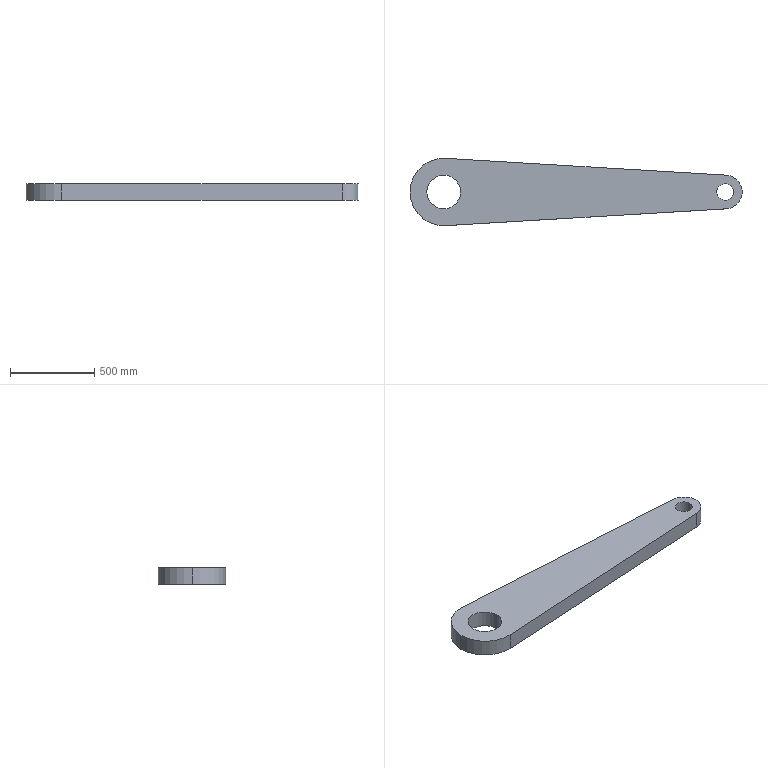Part | SolidWorks | features Extrusion 1 | 1 solid | 11 faces | box 1970 x 400 x 100 mm | volume 54116838 mm3 | cylinder 7 | plane 4 | commonest cylinder face diameters 200 x3 100 x2 400 x2
STEP:
#1=CARTESIAN_POINT('',(1620.,0.,100.));
#2=VERTEX_POINT('',#1);
#3=CARTESIAN_POINT('',(1720.,0.,100.));
#4=VERTEX_POINT('',#3);
#5=CARTESIAN_POINT('',(1670.,0.,100.));
#6=DIRECTION('',(0.,0.,1.));
#7=DIRECTION('',(1.,0.,0.));
#8=AXIS2_PLACEMENT_3D('',#5,#6,#7);
#9=CIRCLE('',#8,50.);
#10=EDGE_CURVE('',#2,#4,#9,.T.);
#11=ORIENTED_EDGE('',*,*,#10,.T.);
#12=CARTESIAN_POINT('',(1720.,0.,0.));
#13=VERTEX_POINT('',#12);
#14=CARTESIAN_POINT('',(1720.,0.,100.));
#15=DIRECTION('',(0.,0.,-1.));
#16=VECTOR('',#15,1000.);
#17=LINE('',#14,#16);
#18=EDGE_CURVE('',#4,#13,#17,.T.);
#19=ORIENTED_EDGE('',*,*,#18,.T.);
#20=CARTESIAN_POINT('',(1620.,0.,0.));
#21=VERTEX_POINT('',#20);
#22=CARTESIAN_POINT('',(1670.,0.,0.));
#23=DIRECTION('',(0.,0.,1.));
#24=DIRECTION('',(1.,0.,0.));
#25=AXIS2_PLACEMENT_3D('',#22,#23,#24);
#26=CIRCLE('',#25,50.);
#27=EDGE_CURVE('',#21,#13,#26,.T.);
#28=ORIENTED_EDGE('',*,*,#27,.F.);
#29=CARTESIAN_POINT('',(1620.,0.,100.));
#30=DIRECTION('',(0.,0.,-1.));
#31=VECTOR('',#30,1000.);
#32=LINE('',#29,#31);
#33=EDGE_CURVE('',#2,#21,#32,.T.);
#34=ORIENTED_EDGE('',*,*,#33,.F.);
#35=EDGE_LOOP('',(#11,#19,#28,#34));
#36=FACE_OUTER_BOUND('',#35,.T.);
#37=CARTESIAN_POINT('',(1670.,0.,100.));
#38=DIRECTION('',(0.,0.,-1.));
#39=DIRECTION('',(-1.,0.,0.));
#40=AXIS2_PLACEMENT_3D('',#37,#38,#39);
#41=CYLINDRICAL_SURFACE('',#40,50.);
#42=ADVANCED_FACE('',(#36),#41,.F.);
#43=CARTESIAN_POINT('',(-100.,0.,100.));
#44=VERTEX_POINT('',#43);
#45=CARTESIAN_POINT('',(100.,0.,100.));
#46=VERTEX_POINT('',#45);
#47=CARTESIAN_POINT('',(0.,0.,100.));
#48=DIRECTION('',(0.,0.,1.));
#49=DIRECTION('',(1.,0.,0.));
#50=AXIS2_PLACEMENT_3D('',#47,#48,#49);
#51=CIRCLE('',#50,100.);
#52=EDGE_CURVE('',#44,#46,#51,.T.);
#53=ORIENTED_EDGE('',*,*,#52,.T.);
#54=CARTESIAN_POINT('',(100.,0.,0.));
#55=VERTEX_POINT('',#54);
#56=CARTESIAN_POINT('',(100.,0.,100.));
#57=DIRECTION('',(0.,0.,-1.));
#58=VECTOR('',#57,1000.);
#59=LINE('',#56,#58);
#60=EDGE_CURVE('',#46,#55,#59,.T.);
#61=ORIENTED_EDGE('',*,*,#60,.T.);
#62=CARTESIAN_POINT('',(-100.,0.,0.));
#63=VERTEX_POINT('',#62);
#64=CARTESIAN_POINT('',(0.,0.,0.));
#65=DIRECTION('',(0.,0.,1.));
#66=DIRECTION('',(1.,0.,0.));
#67=AXIS2_PLACEMENT_3D('',#64,#65,#66);
#68=CIRCLE('',#67,100.);
#69=EDGE_CURVE('',#63,#55,#68,.T.);
#70=ORIENTED_EDGE('',*,*,#69,.F.);
#71=CARTESIAN_POINT('',(-100.,0.,100.));
#72=DIRECTION('',(0.,0.,-1.));
#73=VECTOR('',#72,1000.);
#74=LINE('',#71,#73);
#75=EDGE_CURVE('',#44,#63,#74,.T.);
#76=ORIENTED_EDGE('',*,*,#75,.F.);
#77=EDGE_LOOP('',(#53,#61,#70,#76));
#78=FACE_OUTER_BOUND('',#77,.T.);
#79=CARTESIAN_POINT('',(0.,0.,100.));
#80=DIRECTION('',(0.,0.,-1.));
#81=DIRECTION('',(-1.,0.,0.));
#82=AXIS2_PLACEMENT_3D('',#79,#80,#81);
#83=CYLINDRICAL_SURFACE('',#82,100.);
#84=ADVANCED_FACE('',(#78),#83,.F.);
#85=CARTESIAN_POINT('',(-200.,0.,100.));
#86=VERTEX_POINT('',#85);
#87=CARTESIAN_POINT('',(11.976,-199.641,100.));
#88=VERTEX_POINT('',#87);
#89=CARTESIAN_POINT('',(0.,0.,100.));
#90=DIRECTION('',(0.,0.,1.));
#91=DIRECTION('',(1.,0.,0.));
#92=AXIS2_PLACEMENT_3D('',#89,#90,#91);
#93=CIRCLE('',#92,200.);
#94=EDGE_CURVE('',#86,#88,#93,.T.);
#95=ORIENTED_EDGE('',*,*,#94,.F.);
#96=CARTESIAN_POINT('',(-200.,0.,0.));
#97=VERTEX_POINT('',#96);
#98=CARTESIAN_POINT('',(-200.,0.,100.));
#99=DIRECTION('',(0.,0.,-1.));
#100=VECTOR('',#99,1000.);
#101=LINE('',#98,#100);
#102=EDGE_CURVE('',#86,#97,#101,.T.);
#103=ORIENTED_EDGE('',*,*,#102,.T.);
#104=CARTESIAN_POINT('',(11.976,-199.641,0.));
#105=VERTEX_POINT('',#104);
#106=CARTESIAN_POINT('',(0.,0.,0.));
#107=DIRECTION('',(0.,0.,1.));
#108=DIRECTION('',(1.,0.,0.));
#109=AXIS2_PLACEMENT_3D('',#106,#107,#108);
#110=CIRCLE('',#109,200.);
#111=EDGE_CURVE('',#97,#105,#110,.T.);
#112=ORIENTED_EDGE('',*,*,#111,.T.);
#113=CARTESIAN_POINT('',(11.976,-199.641,100.));
#114=DIRECTION('',(0.,0.,-1.));
#115=VECTOR('',#114,1000.);
#116=LINE('',#113,#115);
#117=EDGE_CURVE('',#88,#105,#116,.T.);
#118=ORIENTED_EDGE('',*,*,#117,.F.);
#119=EDGE_LOOP('',(#95,#103,#112,#118));
#120=FACE_OUTER_BOUND('',#119,.T.);
#121=CARTESIAN_POINT('',(0.,0.,100.));
#122=DIRECTION('',(0.,0.,-1.));
#123=DIRECTION('',(-1.,0.,0.));
#124=AXIS2_PLACEMENT_3D('',#121,#122,#123);
#125=CYLINDRICAL_SURFACE('',#124,200.);
#126=ADVANCED_FACE('',(#120),#125,.T.);
#127=ORIENTED_EDGE('',*,*,#52,.F.);
#128=CARTESIAN_POINT('',(0.,0.,100.));
#129=DIRECTION('',(0.,0.,1.));
#130=DIRECTION('',(1.,0.,0.));
#131=AXIS2_PLACEMENT_3D('',#128,#129,#130);
#132=CIRCLE('',#131,100.);
#133=EDGE_CURVE('',#46,#44,#132,.T.);
#134=ORIENTED_EDGE('',*,*,#133,.F.);
#135=EDGE_LOOP('',(#127,#134));
#136=FACE_BOUND('',#135,.T.);
#137=CARTESIAN_POINT('',(1675.988,-99.821,100.));
#138=VERTEX_POINT('',#137);
#139=CARTESIAN_POINT('',(1675.988,99.821,100.));
#140=VERTEX_POINT('',#139);
#141=CARTESIAN_POINT('',(1670.,0.,100.));
#142=DIRECTION('',(0.,0.,1.));
#143=DIRECTION('',(1.,0.,0.));
#144=AXIS2_PLACEMENT_3D('',#141,#142,#143);
#145=CIRCLE('',#144,100.);
#146=EDGE_CURVE('',#138,#140,#145,.T.);
#147=ORIENTED_EDGE('',*,*,#146,.T.);
#148=CARTESIAN_POINT('',(11.976,199.641,100.));
#149=VERTEX_POINT('',#148);
#150=CARTESIAN_POINT('',(11.976,199.641,100.));
#151=DIRECTION('',(-0.9982,0.05988,0.));
#152=VECTOR('',#151,1000.);
#153=LINE('',#150,#152);
#154=EDGE_CURVE('',#140,#149,#153,.T.);
#155=ORIENTED_EDGE('',*,*,#154,.T.);
#156=CARTESIAN_POINT('',(0.,0.,100.));
#157=DIRECTION('',(0.,0.,1.));
#158=DIRECTION('',(1.,0.,0.));
#159=AXIS2_PLACEMENT_3D('',#156,#157,#158);
#160=CIRCLE('',#159,200.);
#161=EDGE_CURVE('',#149,#86,#160,.T.);
#162=ORIENTED_EDGE('',*,*,#161,.T.);
#163=ORIENTED_EDGE('',*,*,#94,.T.);
#164=CARTESIAN_POINT('',(11.976,-199.641,100.));
#165=DIRECTION('',(0.9982,0.05988,0.));
#166=VECTOR('',#165,1000.);
#167=LINE('',#164,#166);
#168=EDGE_CURVE('',#88,#138,#167,.T.);
#169=ORIENTED_EDGE('',*,*,#168,.T.);
#170=EDGE_LOOP('',(#147,#155,#162,#163,#169));
#171=FACE_OUTER_BOUND('',#170,.T.);
#172=ORIENTED_EDGE('',*,*,#10,.F.);
#173=CARTESIAN_POINT('',(1670.,0.,100.));
#174=DIRECTION('',(0.,0.,1.));
#175=DIRECTION('',(1.,0.,0.));
#176=AXIS2_PLACEMENT_3D('',#173,#174,#175);
#177=CIRCLE('',#176,50.);
#178=EDGE_CURVE('',#4,#2,#177,.T.);
#179=ORIENTED_EDGE('',*,*,#178,.F.);
#180=EDGE_LOOP('',(#172,#179));
#181=FACE_BOUND('',#180,.T.);
#182=CARTESIAN_POINT('',(1670.,0.,100.));
#183=DIRECTION('',(0.,0.,1.));
#184=DIRECTION('',(1.,0.,0.));
#185=AXIS2_PLACEMENT_3D('',#182,#183,#184);
#186=PLANE('',#185);
#187=ADVANCED_FACE('',(#136,#171,#181),#186,.T.);
#188=ORIENTED_EDGE('',*,*,#69,.T.);
#189=CARTESIAN_POINT('',(0.,0.,0.));
#190=DIRECTION('',(0.,0.,1.));
#191=DIRECTION('',(1.,0.,0.));
#192=AXIS2_PLACEMENT_3D('',#189,#190,#191);
#193=CIRCLE('',#192,100.);
#194=EDGE_CURVE('',#55,#63,#193,.T.);
#195=ORIENTED_EDGE('',*,*,#194,.T.);
#196=EDGE_LOOP('',(#188,#195));
#197=FACE_BOUND('',#196,.T.);
#198=CARTESIAN_POINT('',(1675.988,-99.821,0.));
#199=VERTEX_POINT('',#198);
#200=CARTESIAN_POINT('',(1675.988,99.821,0.));
#201=VERTEX_POINT('',#200);
#202=CARTESIAN_POINT('',(1670.,0.,0.));
#203=DIRECTION('',(0.,0.,1.));
#204=DIRECTION('',(1.,0.,0.));
#205=AXIS2_PLACEMENT_3D('',#202,#203,#204);
#206=CIRCLE('',#205,100.);
#207=EDGE_CURVE('',#199,#201,#206,.T.);
#208=ORIENTED_EDGE('',*,*,#207,.F.);
#209=CARTESIAN_POINT('',(11.976,-199.641,0.));
#210=DIRECTION('',(0.9982,0.05988,0.));
#211=VECTOR('',#210,1000.);
#212=LINE('',#209,#211);
#213=EDGE_CURVE('',#105,#199,#212,.T.);
#214=ORIENTED_EDGE('',*,*,#213,.F.);
#215=ORIENTED_EDGE('',*,*,#111,.F.);
#216=CARTESIAN_POINT('',(11.976,199.641,0.));
#217=VERTEX_POINT('',#216);
#218=CARTESIAN_POINT('',(0.,0.,0.));
#219=DIRECTION('',(0.,0.,1.));
#220=DIRECTION('',(1.,0.,0.));
#221=AXIS2_PLACEMENT_3D('',#218,#219,#220);
#222=CIRCLE('',#221,200.);
#223=EDGE_CURVE('',#217,#97,#222,.T.);
#224=ORIENTED_EDGE('',*,*,#223,.F.);
#225=CARTESIAN_POINT('',(11.976,199.641,0.));
#226=DIRECTION('',(-0.9982,0.05988,0.));
#227=VECTOR('',#226,1000.);
#228=LINE('',#225,#227);
#229=EDGE_CURVE('',#201,#217,#228,.T.);
#230=ORIENTED_EDGE('',*,*,#229,.F.);
#231=EDGE_LOOP('',(#208,#214,#215,#224,#230));
#232=FACE_OUTER_BOUND('',#231,.T.);
#233=ORIENTED_EDGE('',*,*,#27,.T.);
#234=CARTESIAN_POINT('',(1670.,0.,0.));
#235=DIRECTION('',(0.,0.,1.));
#236=DIRECTION('',(1.,0.,0.));
#237=AXIS2_PLACEMENT_3D('',#234,#235,#236);
#238=CIRCLE('',#237,50.);
#239=EDGE_CURVE('',#13,#21,#238,.T.);
#240=ORIENTED_EDGE('',*,*,#239,.T.);
#241=EDGE_LOOP('',(#233,#240));
#242=FACE_BOUND('',#241,.T.);
#243=CARTESIAN_POINT('',(1670.,0.,0.));
#244=DIRECTION('',(0.,0.,1.));
#245=DIRECTION('',(1.,0.,0.));
#246=AXIS2_PLACEMENT_3D('',#243,#244,#245);
#247=PLANE('',#246);
#248=ADVANCED_FACE('',(#197,#232,#242),#247,.F.);
#249=ORIENTED_EDGE('',*,*,#207,.T.);
#250=CARTESIAN_POINT('',(1675.988,99.821,100.));
#251=DIRECTION('',(0.,0.,-1.));
#252=VECTOR('',#251,1000.);
#253=LINE('',#250,#252);
#254=EDGE_CURVE('',#140,#201,#253,.T.);
#255=ORIENTED_EDGE('',*,*,#254,.F.);
#256=ORIENTED_EDGE('',*,*,#146,.F.);
#257=CARTESIAN_POINT('',(1675.988,-99.821,100.));
#258=DIRECTION('',(0.,0.,-1.));
#259=VECTOR('',#258,1000.);
#260=LINE('',#257,#259);
#261=EDGE_CURVE('',#138,#199,#260,.T.);
#262=ORIENTED_EDGE('',*,*,#261,.T.);
#263=EDGE_LOOP('',(#249,#255,#256,#262));
#264=FACE_OUTER_BOUND('',#263,.T.);
#265=CARTESIAN_POINT('',(1670.,0.,100.));
#266=DIRECTION('',(0.,0.,-1.));
#267=DIRECTION('',(-1.,0.,0.));
#268=AXIS2_PLACEMENT_3D('',#265,#266,#267);
#269=CYLINDRICAL_SURFACE('',#268,100.);
#270=ADVANCED_FACE('',(#264),#269,.T.);
#271=ORIENTED_EDGE('',*,*,#229,.T.);
#272=CARTESIAN_POINT('',(11.976,199.641,100.));
#273=DIRECTION('',(0.,0.,-1.));
#274=VECTOR('',#273,1000.);
#275=LINE('',#272,#274);
#276=EDGE_CURVE('',#149,#217,#275,.T.);
#277=ORIENTED_EDGE('',*,*,#276,.F.);
#278=ORIENTED_EDGE('',*,*,#154,.F.);
#279=ORIENTED_EDGE('',*,*,#254,.T.);
#280=EDGE_LOOP('',(#271,#277,#278,#279));
#281=FACE_OUTER_BOUND('',#280,.T.);
#282=CARTESIAN_POINT('',(11.976,199.641,100.));
#283=DIRECTION('',(-0.05988,-0.9982,0.));
#284=DIRECTION('',(0.9982,-0.05988,0.));
#285=AXIS2_PLACEMENT_3D('',#282,#283,#284);
#286=PLANE('',#285);
#287=ADVANCED_FACE('',(#281),#286,.F.);
#288=ORIENTED_EDGE('',*,*,#102,.F.);
#289=ORIENTED_EDGE('',*,*,#161,.F.);
#290=ORIENTED_EDGE('',*,*,#276,.T.);
#291=ORIENTED_EDGE('',*,*,#223,.T.);
#292=EDGE_LOOP('',(#288,#289,#290,#291));
#293=FACE_OUTER_BOUND('',#292,.T.);
#294=CARTESIAN_POINT('',(0.,0.,100.));
#295=DIRECTION('',(0.,0.,-1.));
#296=DIRECTION('',(-1.,0.,0.));
#297=AXIS2_PLACEMENT_3D('',#294,#295,#296);
#298=CYLINDRICAL_SURFACE('',#297,200.);
#299=ADVANCED_FACE('',(#293),#298,.T.);
#300=ORIENTED_EDGE('',*,*,#213,.T.);
#301=ORIENTED_EDGE('',*,*,#261,.F.);
#302=ORIENTED_EDGE('',*,*,#168,.F.);
#303=ORIENTED_EDGE('',*,*,#117,.T.);
#304=EDGE_LOOP('',(#300,#301,#302,#303));
#305=FACE_OUTER_BOUND('',#304,.T.);
#306=CARTESIAN_POINT('',(11.976,-199.641,100.));
#307=DIRECTION('',(-0.05988,0.9982,0.));
#308=DIRECTION('',(-0.9982,-0.05988,0.));
#309=AXIS2_PLACEMENT_3D('',#306,#307,#308);
#310=PLANE('',#309);
#311=ADVANCED_FACE('',(#305),#310,.F.);
#312=ORIENTED_EDGE('',*,*,#60,.F.);
#313=ORIENTED_EDGE('',*,*,#133,.T.);
#314=ORIENTED_EDGE('',*,*,#75,.T.);
#315=ORIENTED_EDGE('',*,*,#194,.F.);
#316=EDGE_LOOP('',(#312,#313,#314,#315));
#317=FACE_OUTER_BOUND('',#316,.T.);
#318=CARTESIAN_POINT('',(0.,0.,100.));
#319=DIRECTION('',(0.,0.,-1.));
#320=DIRECTION('',(-1.,0.,0.));
#321=AXIS2_PLACEMENT_3D('',#318,#319,#320);
#322=CYLINDRICAL_SURFACE('',#321,100.);
#323=ADVANCED_FACE('',(#317),#322,.F.);
#324=ORIENTED_EDGE('',*,*,#18,.F.);
#325=ORIENTED_EDGE('',*,*,#178,.T.);
#326=ORIENTED_EDGE('',*,*,#33,.T.);
#327=ORIENTED_EDGE('',*,*,#239,.F.);
#328=EDGE_LOOP('',(#324,#325,#326,#327));
#329=FACE_OUTER_BOUND('',#328,.T.);
#330=CARTESIAN_POINT('',(1670.,0.,100.));
#331=DIRECTION('',(0.,0.,-1.));
#332=DIRECTION('',(-1.,0.,0.));
#333=AXIS2_PLACEMENT_3D('',#330,#331,#332);
#334=CYLINDRICAL_SURFACE('',#333,50.);
#335=ADVANCED_FACE('',(#329),#334,.F.);
#336=CLOSED_SHELL('',(#42,#84,#126,#187,#248,#270,#287,#299,#311,#323,#335));
#337=MANIFOLD_SOLID_BREP('',#336);
#338=CARTESIAN_POINT('',(0.,0.,0.));
#339=DIRECTION('',(0.,0.,1.));
#340=DIRECTION('',(1.,0.,0.));
#341=AXIS2_PLACEMENT_3D('',#338,#339,#340);
#342=(LENGTH_UNIT()NAMED_UNIT(*)SI_UNIT(.MILLI.,.METRE.));
#343=UNCERTAINTY_MEASURE_WITH_UNIT(LENGTH_MEASURE(0.00001),#342,'','');
#344=(NAMED_UNIT(*)PLANE_ANGLE_UNIT()SI_UNIT($,.RADIAN.));
#345=(NAMED_UNIT(*)SI_UNIT($,.STERADIAN.)SOLID_ANGLE_UNIT());
#346=(GEOMETRIC_REPRESENTATION_CONTEXT(3)GLOBAL_UNCERTAINTY_ASSIGNED_CONTEXT((#343))GLOBAL_UNIT_ASSIGNED_CONTEXT((#342,#344,#345))REPRESENTATION_CONTEXT('',''));
#347=ADVANCED_BREP_SHAPE_REPRESENTATION('',(#337,#341),#346);